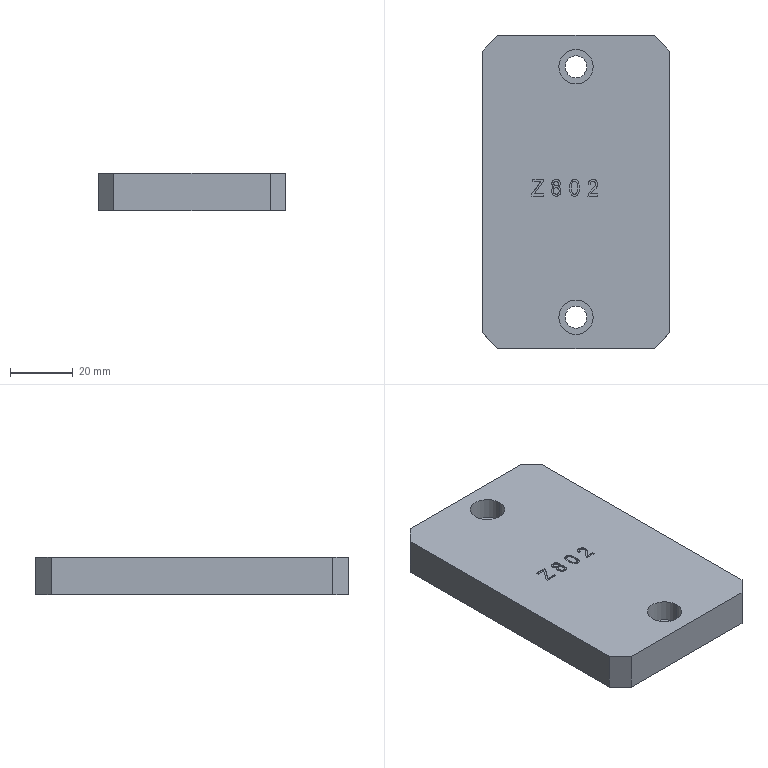Part | Creo | 1 solid | 114 faces | box 60 x 100 x 12 mm | volume 69679 mm3 | other 73 | plane 30 | cylinder 11 | commonest cylinder face diameters 7 x4 11 x4 2.625 x1 4.553 x1 71.806 x1